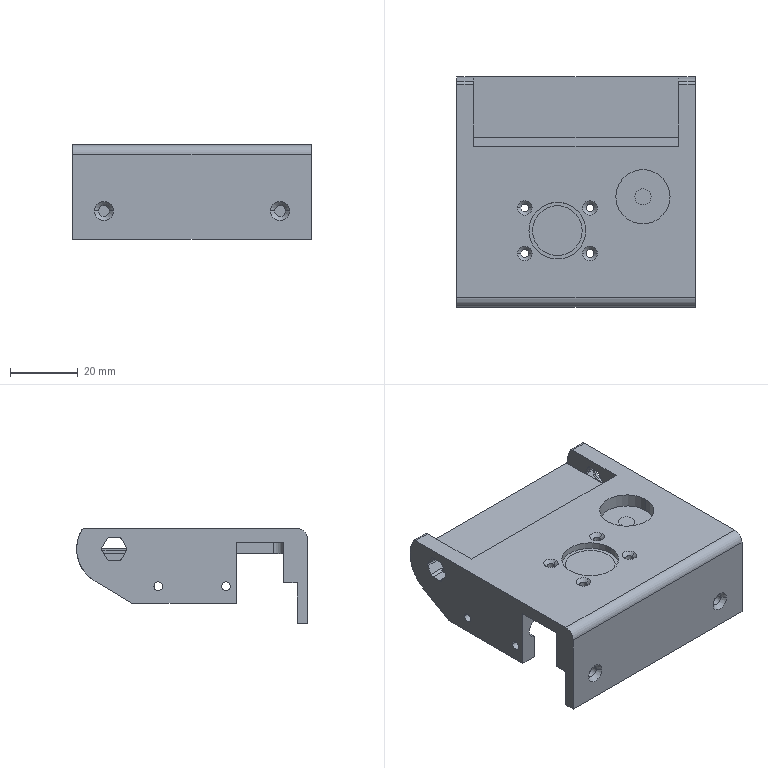NC program | NX | posted with a generic post | part box 70.5 x 68.1 x 28 mm
Whole program:
N10 G17 G21 G94 G90
(DRILLING_COPY_1 , TOOL : D6A45)
N12 T07 M6
N14 G54
N16 G17 G0 G90 X-24. Y-17. B0. C0. S3500 M3
N18 G43 Z30. H7
N20 G94 G81 G98 Z-1.4 F250. R3.
N22 X-44.
N24 G80
N26 G0 X-44. Y-17. Z30.
N28 M5
(DRILLING_COPY_COPY_COPY_1 , TOOL : 2.6ZT)
N30 T12 M6
N32 G54
N34 G17 G0 G90 X-24. Y-17. B0. C0. S2500 M3
N36 G43 Z30. H12
N38 G94 G83 G98 Z-7.281 F120. Q2. R3.
N40 X-44.
N42 G80
N44 G0 X-44. Y-17. Z30.
N46 M5
(ZLEVEL_PROFILE_COPY , TOOL : D2)
N48 T02 M6
N50 G54
N52 G17 G0 G90 X-55.895 Y-3.6 B0. C0. S9500 M3
N54 G43 Z30. H2
N56 Z1.
N58 G94 G1 X-58.386 Z0.869 F1000.
N60 X-59.769 Y-5.996 Z0.724
N62 X-59.764 Y-5.999
N64 X-59.765 Y-6.012
N66 X-58.388 Y-8.396 Z0.579
N68 X-58.379 Y-8.4
N70 X-55.614 Z0.434
N72 X-54.232 Y-6.006 Z0.289
N74 X-54.231 Y-5.996 Z0.288
N76 X-55.614 Y-3.6 Z0.143
N78 X-58.386 Z-0.002
N80 X-59.769 Y-5.996 Z-0.147
N82 X-59.764 Y-5.999
N84 X-59.765 Y-6.012
N86 X-58.388 Y-8.396
N88 X-58.379 Y-8.4
N90 X-55.614
N92 X-54.232 Y-6.006
N94 X-54.231 Y-5.996
N96 X-55.614 Y-3.6
N98 X-58.386
N100 X-59.769 Y-5.996
N102 X-59.764 Y-5.999
N104 X-59.721 Y-6.087 Z-0.149
N106 X-59.673 Y-6.17 Z-0.15
N108 X-58.448 Y-8.291 Z-0.193
N110 X-58.396 Y-8.374 Z-0.195
N112 X-58.376 Y-8.394
N114 X-58.216 Y-8.4 Z-0.198
N116 X-55.669 Z-0.243
N118 X-55.619 Y-8.393 Z-0.244
N120 X-55.543 Y-8.277 Z-0.246
N122 X-54.27 Y-6.071 Z-0.291
N124 X-54.248 Y-6.029 Z-0.292
N126 X-54.237 Y-5.986
N128 X-54.286 Y-5.9 Z-0.294
N130 X-55.614 Y-3.6
N132 X-58.386
N134 X-59.769 Y-5.996
N136 X-59.764 Y-5.999
N138 X-59.721 Y-6.087 Z-0.296
N140 X-59.673 Y-6.17 Z-0.298
N142 X-58.448 Y-8.291 Z-0.34
N144 X-58.396 Y-8.374 Z-0.342
N146 X-58.376 Y-8.394 Z-0.343
N148 X-58.216 Y-8.4 Z-0.345
N150 X-55.669 Z-0.39
N152 X-55.619 Y-8.393 Z-0.391
N154 X-55.543 Y-8.277 Z-0.393
N156 X-54.27 Y-6.071 Z-0.438
N158 X-54.248 Y-6.029 Z-0.439
N160 X-54.237 Y-5.986
N162 X-54.286 Y-5.9 Z-0.441
N164 X-55.614 Y-3.6
N166 X-58.386
N168 X-59.769 Y-5.996
N170 X-59.764 Y-5.999
N172 X-59.721 Y-6.087 Z-0.443
N174 X-59.673 Y-6.17 Z-0.445
N176 X-58.448 Y-8.291 Z-0.487
N178 X-58.396 Y-8.374 Z-0.489
N180 X-58.376 Y-8.394 Z-0.49
N182 X-58.216 Y-8.4 Z-0.492
N184 X-55.669 Z-0.537
N186 X-55.619 Y-8.392 Z-0.538
N188 X-55.543 Y-8.277 Z-0.54
N190 X-54.27 Y-6.071 Z-0.585
N192 X-54.248 Y-6.029 Z-0.586
N194 X-54.237 Y-5.986 Z-0.587
N196 X-54.286 Y-5.9 Z-0.588
N198 X-55.614 Y-3.6
N200 X-58.386
N202 X-59.769 Y-5.996
N204 X-59.764 Y-5.999
N206 X-59.721 Y-6.087 Z-0.59
N208 X-59.673 Y-6.17 Z-0.592
N210 X-58.448 Y-8.291 Z-0.634
N212 X-58.396 Y-8.374 Z-0.636
N214 X-58.376 Y-8.394 Z-0.637
N216 X-58.216 Y-8.4 Z-0.64
N218 X-55.669 Z-0.684
N220 X-55.619 Y-8.392 Z-0.685
N222 X-55.543 Y-8.277 Z-0.687
N224 X-54.27 Y-6.071 Z-0.732
N226 X-54.248 Y-6.029 Z-0.733
N228 X-54.237 Y-5.986 Z-0.734
N230 X-54.286 Y-5.9 Z-0.735
N232 X-55.614 Y-3.6
N234 X-58.386
N236 X-59.769 Y-5.996
N238 X-59.764 Y-5.999
N240 X-59.721 Y-6.087 Z-0.737
N242 X-59.673 Y-6.17 Z-0.739
N244 X-58.448 Y-8.291 Z-0.781
N246 X-58.396 Y-8.374 Z-0.783
N248 X-58.376 Y-8.394 Z-0.784
N250 X-58.216 Y-8.4 Z-0.787
N252 X-55.669 Z-0.831
N254 X-55.619 Y-8.392 Z-0.832
N256 X-55.543 Y-8.277 Z-0.834
N258 X-54.27 Y-6.071 Z-0.879
N260 X-54.248 Y-6.029 Z-0.88
N262 X-54.237 Y-5.986 Z-0.881
N264 X-54.286 Y-5.9 Z-0.882
N266 X-55.614 Y-3.6
N268 X-58.386
N270 X-59.769 Y-5.996
N272 X-59.764 Y-5.999
N274 X-59.721 Y-6.087 Z-0.884
N276 X-59.673 Y-6.17 Z-0.886
N278 X-58.448 Y-8.291 Z-0.929
N280 X-58.396 Y-8.374 Z-0.93
N282 X-58.376 Y-8.394 Z-0.931
N284 X-58.216 Y-8.4 Z-0.934
N286 X-55.669 Z-0.978
N288 X-55.619 Y-8.392 Z-0.979
N290 X-55.543 Y-8.277 Z-0.982
N292 X-54.27 Y-6.071 Z-1.026
N294 X-54.248 Y-6.029 Z-1.027
N296 X-54.237 Y-5.986 Z-1.028
N298 X-54.286 Y-5.9 Z-1.029
N300 X-55.614 Y-3.6
N302 X-58.386
N304 X-59.769 Y-5.996
N306 X-59.764 Y-5.999
N308 X-59.721 Y-6.087 Z-1.031
N310 X-59.673 Y-6.17 Z-1.033
N312 X-58.448 Y-8.291 Z-1.076
N314 X-58.396 Y-8.374 Z-1.077
N316 X-58.376 Y-8.394 Z-1.078
N318 X-58.216 Y-8.4 Z-1.081
N320 X-55.669 Z-1.125
N322 X-55.619 Y-8.392 Z-1.126
N324 X-55.543 Y-8.277 Z-1.129
N326 X-54.27 Y-6.071 Z-1.173
N328 X-54.248 Y-6.029 Z-1.174
N330 X-54.237 Y-5.986 Z-1.175
N332 X-54.286 Y-5.9 Z-1.176
N334 X-55.614 Y-3.6
N336 X-58.386
N338 X-59.769 Y-5.996
N340 X-59.764 Y-5.999
N342 X-59.721 Y-6.087 Z-1.178
N344 X-59.673 Y-6.17 Z-1.18
N346 X-58.448 Y-8.291 Z-1.223
N348 X-58.396 Y-8.374 Z-1.224
N350 X-58.376 Y-8.394 Z-1.225
N352 X-58.216 Y-8.4 Z-1.228
N354 X-55.669 Z-1.272
N356 X-55.619 Y-8.392 Z-1.273
N358 X-55.543 Y-8.277 Z-1.276
N360 X-54.27 Y-6.071 Z-1.32
N362 X-54.248 Y-6.029 Z-1.321
N364 X-54.237 Y-5.986 Z-1.322
N366 X-54.286 Y-5.9 Z-1.324
N368 X-55.614 Y-3.6
N370 X-58.386
N372 X-59.769 Y-5.996
N374 X-59.764 Y-5.999
N376 X-59.721 Y-6.087 Z-1.325
N378 X-59.673 Y-6.17 Z-1.327
N380 X-58.448 Y-8.291 Z-1.37
N382 X-58.396 Y-8.374 Z-1.371
N384 X-58.376 Y-8.394 Z-1.372
N386 X-58.216 Y-8.4 Z-1.375
N388 X-55.669 Z-1.419
N390 X-55.619 Y-8.392 Z-1.42
N392 X-55.543 Y-8.277 Z-1.423
N394 X-54.27 Y-6.071 Z-1.467
N396 X-54.248 Y-6.029 Z-1.468
N398 X-54.237 Y-5.986 Z-1.469
N400 X-54.286 Y-5.9 Z-1.471
N402 X-55.614 Y-3.6
N404 X-58.386
N406 X-59.769 Y-5.996
N408 X-59.764 Y-5.999
N410 X-59.721 Y-6.087 Z-1.472
N412 X-59.673 Y-6.17 Z-1.474
N414 X-58.448 Y-8.291 Z-1.517
N416 X-58.396 Y-8.374 Z-1.518
N418 X-58.376 Y-8.394 Z-1.519
N420 X-58.216 Y-8.4 Z-1.522
N422 X-55.669 Z-1.566
N424 X-55.619 Y-8.392 Z-1.567
N426 X-55.543 Y-8.277 Z-1.57
N428 X-54.27 Y-6.071 Z-1.614
N430 X-54.248 Y-6.029 Z-1.615
N432 X-54.237 Y-5.986 Z-1.616
N434 X-54.287 Y-5.9 Z-1.618
N436 X-55.614 Y-3.6
N438 X-58.386
N440 X-59.769 Y-5.996
N442 X-59.764 Y-5.999
N444 X-59.721 Y-6.087 Z-1.619
N446 X-59.673 Y-6.17 Z-1.621
N448 X-58.448 Y-8.291 Z-1.664
N450 X-58.396 Y-8.374 Z-1.666
N452 X-58.376 Y-8.393
N454 X-58.216 Y-8.4 Z-1.669
N456 X-55.669 Z-1.713
N458 X-55.619 Y-8.392 Z-1.714
N460 X-55.543 Y-8.277 Z-1.717
N462 X-54.27 Y-6.071 Z-1.761
N464 X-54.248 Y-6.029 Z-1.762
N466 X-54.237 Y-5.986 Z-1.763
N468 X-54.287 Y-5.9 Z-1.765
N470 X-55.614 Y-3.6
N472 X-58.386
N474 X-59.769 Y-5.996
N476 X-59.764 Y-5.999
N478 X-59.721 Y-6.087 Z-1.766
N480 X-59.673 Y-6.17 Z-1.768
N482 X-58.448 Y-8.291 Z-1.811
N484 X-58.396 Y-8.374 Z-1.813
N486 X-58.376 Y-8.393
N488 X-58.216 Y-8.4 Z-1.816
N490 X-55.669 Z-1.86
N492 X-55.619 Y-8.392 Z-1.861
N494 X-55.543 Y-8.277 Z-1.864
N496 X-54.27 Y-6.071 Z-1.908
N498 X-54.248 Y-6.029 Z-1.909
N500 X-54.237 Y-5.986 Z-1.91
N502 X-54.287 Y-5.9 Z-1.912
N504 X-55.614 Y-3.6
N506 X-58.386
N508 X-59.769 Y-5.996
N510 X-59.764 Y-5.999
N512 X-59.721 Y-6.087 Z-1.913
N514 X-59.673 Y-6.17 Z-1.915
N516 X-58.448 Y-8.291 Z-1.958
N518 X-58.396 Y-8.374 Z-1.96
N520 X-58.376 Y-8.393
N522 X-58.216 Y-8.4 Z-1.963
N524 X-55.669 Z-2.008
N526 X-55.619 Y-8.392
N528 X-55.543 Y-8.277 Z-2.011
N530 X-54.27 Y-6.071 Z-2.055
N532 X-54.248 Y-6.029 Z-2.056
N534 X-54.237 Y-5.986 Z-2.057
N536 X-54.287 Y-5.9 Z-2.059
N538 X-55.614 Y-3.6
N540 X-58.386
N542 X-59.769 Y-5.996
N544 X-59.764 Y-5.999
N546 X-59.721 Y-6.087 Z-2.061
N548 X-59.673 Y-6.17 Z-2.062
N550 X-58.448 Y-8.291 Z-2.105
N552 X-58.396 Y-8.374 Z-2.107
N554 X-58.376 Y-8.393
N556 X-58.216 Y-8.4 Z-2.11
N558 X-55.669 Z-2.155
N560 X-55.619 Y-8.392 Z-2.156
N562 X-55.543 Y-8.277 Z-2.158
N564 X-54.27 Y-6.071 Z-2.202
N566 X-54.248 Y-6.029 Z-2.203
N568 X-54.237 Y-5.986 Z-2.204
N570 X-54.287 Y-5.9 Z-2.206
N572 X-55.614 Y-3.6
N574 X-58.386
N576 X-59.769 Y-5.996
N578 X-59.764 Y-5.999
N580 X-59.721 Y-6.087 Z-2.208
N582 X-59.673 Y-6.17 Z-2.209
N584 X-58.448 Y-8.291 Z-2.252
N586 X-58.396 Y-8.374 Z-2.254
N588 X-58.376 Y-8.393
N590 X-58.216 Y-8.4 Z-2.257
N592 X-55.669 Z-2.302
N594 X-55.619 Y-8.392 Z-2.303
N596 X-55.543 Y-8.277 Z-2.305
N598 X-54.27 Y-6.071 Z-2.35
N600 X-54.248 Y-6.029
N602 X-54.237 Y-5.986 Z-2.351
N604 X-54.287 Y-5.9 Z-2.353
N606 X-55.614 Y-3.6
N608 X-58.386
N610 X-59.769 Y-5.996
N612 X-59.764 Y-5.999
N614 X-59.721 Y-6.087 Z-2.355
N616 X-59.673 Y-6.17 Z-2.356
N618 X-58.448 Y-8.291 Z-2.399
N620 X-58.396 Y-8.374 Z-2.401
N622 X-58.376 Y-8.393
N624 X-58.216 Y-8.4 Z-2.404
N626 X-55.669 Z-2.449
N628 X-55.619 Y-8.392 Z-2.45
N630 X-55.543 Y-8.277 Z-2.452
N632 X-54.27 Y-6.071 Z-2.497
N634 X-54.248 Y-6.029
N636 X-54.237 Y-5.986 Z-2.498
N638 X-54.287 Y-5.9 Z-2.5
N640 X-55.614 Y-3.6
N642 X-58.386
N644 X-59.769 Y-5.996
N646 X-59.764 Y-5.999
N648 X-59.721 Y-6.087 Z-2.502
N650 X-59.673 Y-6.17 Z-2.503
N652 X-58.448 Y-8.291 Z-2.546
N654 X-58.396 Y-8.374 Z-2.548
N656 X-58.376 Y-8.393
N658 X-58.216 Y-8.4 Z-2.551
N660 X-55.669 Z-2.596
N662 X-55.619 Y-8.392 Z-2.597
N664 X-55.543 Y-8.277 Z-2.599
N666 X-54.27 Y-6.071 Z-2.644
N668 X-54.248 Y-6.029
N670 X-54.237 Y-5.986 Z-2.645
N672 X-54.287 Y-5.9 Z-2.647
N674 X-55.614 Y-3.6
N676 X-58.386
N678 X-59.769 Y-5.996
N680 X-59.764 Y-5.999
N682 X-59.721 Y-6.087 Z-2.649
N684 X-59.673 Y-6.17 Z-2.65
N686 X-58.448 Y-8.291 Z-2.693
N688 X-58.396 Y-8.374 Z-2.695
N690 X-58.376 Y-8.393
N692 X-58.216 Y-8.4 Z-2.698
N694 X-55.669 Z-2.743
N696 X-55.619 Y-8.392 Z-2.744
N698 X-55.543 Y-8.277 Z-2.746
N700 X-54.27 Y-6.071 Z-2.791
N702 X-54.248 Y-6.029 Z-2.792
N704 X-54.237 Y-5.986
N706 X-54.287 Y-5.9 Z-2.794
N708 X-55.614 Y-3.6
N710 X-58.386
N712 X-59.769 Y-5.996
N714 X-59.764 Y-5.999
N716 X-59.721 Y-6.087 Z-2.796
N718 X-59.673 Y-6.17 Z-2.798
N720 X-58.448 Y-8.291 Z-2.84
N722 X-58.396 Y-8.374 Z-2.842
N724 X-58.376 Y-8.393 Z-2.843
N726 X-58.216 Y-8.4 Z-2.845
N728 X-55.669 Z-2.89
N730 X-55.619 Y-8.392 Z-2.891
N732 X-55.543 Y-8.277 Z-2.893
N734 X-54.27 Y-6.071 Z-2.938
N736 X-54.248 Y-6.029 Z-2.939
N738 X-54.237 Y-5.986
N740 X-54.287 Y-5.9 Z-2.941
N742 X-55.614 Y-3.6
N744 X-58.386
N746 X-59.769 Y-5.996
N748 X-59.764 Y-5.999
N750 X-59.721 Y-6.087 Z-2.943
N752 X-59.673 Y-6.17 Z-2.945
N754 X-58.448 Y-8.291 Z-2.987
N756 X-58.396 Y-8.374 Z-2.989
N758 X-58.376 Y-8.393 Z-2.99
N760 X-58.216 Y-8.4 Z-2.992
N762 X-55.669 Z-3.037
N764 X-55.619 Y-8.392 Z-3.038
N766 X-55.543 Y-8.277 Z-3.04
N768 X-54.27 Y-6.071 Z-3.085
N770 X-54.248 Y-6.029 Z-3.086
N772 X-54.237 Y-5.986 Z-3.087
N774 X-54.287 Y-5.9 Z-3.088
N776 X-55.614 Y-3.6
N778 X-58.386
N780 X-59.769 Y-5.996
N782 X-59.764 Y-5.999
N784 X-59.721 Y-6.087 Z-3.09
N786 X-59.673 Y-6.17 Z-3.092
N788 X-58.448 Y-8.291 Z-3.134
N790 X-58.396 Y-8.374 Z-3.136
N792 X-58.376 Y-8.393 Z-3.137
N794 X-58.216 Y-8.4 Z-3.14
N796 X-55.669 Z-3.184
N798 X-55.619 Y-8.392 Z-3.185
N800 X-55.543 Y-8.277 Z-3.187
N802 X-54.27 Y-6.071 Z-3.232
N804 X-54.248 Y-6.029 Z-3.233
N806 X-54.237 Y-5.986 Z-3.234
N808 X-54.287 Y-5.9 Z-3.235
N810 X-55.614 Y-3.6
N812 X-58.386
N814 X-59.769 Y-5.996
N816 X-59.764 Y-5.999
N818 X-59.721 Y-6.087 Z-3.237
N820 X-59.673 Y-6.17 Z-3.239
N822 X-58.448 Y-8.291 Z-3.281
N824 X-58.396 Y-8.374 Z-3.283
N826 X-58.376 Y-8.393 Z-3.284
N828 X-58.216 Y-8.4 Z-3.287
N830 X-55.669 Z-3.331
N832 X-55.619 Y-8.392 Z-3.332
N834 X-55.543 Y-8.277 Z-3.334
N836 X-54.27 Y-6.071 Z-3.379
N838 X-54.248 Y-6.029 Z-3.38
N840 X-54.237 Y-5.986 Z-3.381
N842 X-54.287 Y-5.9 Z-3.382
N844 X-55.614 Y-3.6
N846 X-58.386
N848 X-59.769 Y-5.996
N850 X-59.764 Y-5.999
N852 X-59.721 Y-6.087 Z-3.384
N854 X-59.673 Y-6.17 Z-3.386
N856 X-58.448 Y-8.291 Z-3.429
N858 X-58.396 Y-8.374 Z-3.43
N860 X-58.376 Y-8.393 Z-3.431
N862 X-58.216 Y-8.4 Z-3.434
N864 X-55.669 Z-3.478
N866 X-55.619 Y-8.391 Z-3.479
N868 X-55.59 Y-8.358 Z-3.48
N870 X-55.542 Y-8.274 Z-3.482
N872 X-54.268 Y-6.068 Z-3.526
N874 X-54.247 Y-6.025 Z-3.527
N876 X-54.239 Y-5.982 Z-3.528
N878 X-54.288 Y-5.897 Z-3.529
N880 X-55.614 Y-3.6
N882 X-58.386
N884 X-59.769 Y-5.996
N886 X-59.764 Y-5.999
N888 X-59.721 Y-6.087 Z-3.531
N890 X-59.673 Y-6.17 Z-3.533
N892 X-58.448 Y-8.291 Z-3.576
N894 X-58.396 Y-8.374 Z-3.577
N896 X-58.376 Y-8.393 Z-3.578
N898 X-58.216 Y-8.4 Z-3.581
N900 X-55.669 Z-3.625
N902 X-55.619 Y-8.391 Z-3.626
N904 X-55.59 Y-8.358 Z-3.627
N906 X-55.542 Y-8.274 Z-3.629
N908 X-54.268 Y-6.068 Z-3.673
N910 X-54.247 Y-6.025 Z-3.674
N912 X-54.239 Y-5.982 Z-3.675
N914 X-54.288 Y-5.897 Z-3.676
N916 X-55.614 Y-3.6
N918 X-58.386
N920 X-59.769 Y-5.996
N922 X-59.764 Y-5.999
N924 X-59.721 Y-6.087 Z-3.678
N926 X-59.673 Y-6.17 Z-3.68
N928 X-58.448 Y-8.291 Z-3.723
N930 X-58.396 Y-8.374 Z-3.724
N932 X-58.376 Y-8.393 Z-3.725
N934 X-58.216 Y-8.4 Z-3.728
N936 X-55.669 Z-3.772
N938 X-55.619 Y-8.391 Z-3.773
N940 X-55.59 Y-8.358 Z-3.774
N942 X-55.542 Y-8.274 Z-3.776
N944 X-54.268 Y-6.068 Z-3.82
N946 X-54.247 Y-6.025 Z-3.821
N948 X-54.239 Y-5.982 Z-3.822
N950 X-54.288 Y-5.897 Z-3.824
N952 X-55.614 Y-3.6
N954 X-58.386
N956 X-59.769 Y-5.996
N958 X-59.764 Y-5.999
N960 X-59.721 Y-6.087 Z-3.825
N962 X-59.673 Y-6.17 Z-3.827
N964 X-58.448 Y-8.291 Z-3.87
N966 X-58.396 Y-8.374 Z-3.871
N968 X-58.375 Y-8.393 Z-3.872
N970 X-58.216 Y-8.4 Z-3.875
N972 X-55.669 Z-3.919
N974 X-55.619 Y-8.391 Z-3.92
N976 X-55.59 Y-8.358 Z-3.921
N978 X-55.542 Y-8.274 Z-3.923
N980 X-54.268 Y-6.068 Z-3.967
N982 X-54.247 Y-6.025 Z-3.968
N984 X-54.239 Y-5.982 Z-3.969
N986 X-54.288 Y-5.897 Z-3.971
N988 X-55.614 Y-3.6
N990 X-58.386
N992 X-59.769 Y-5.996
N994 X-59.764 Y-5.999
N996 X-59.721 Y-6.087 Z-3.972
N998 X-59.673 Y-6.17 Z-3.974
N1000 X-58.448 Y-8.291 Z-4.017
N1002 X-58.396 Y-8.374 Z-4.018
N1004 X-58.375 Y-8.393 Z-4.019
N1006 X-58.215 Y-8.4 Z-4.022
N1008 X-55.668 Z-4.066
N1010 X-55.619 Y-8.391 Z-4.067
N1012 X-55.591 Y-8.359 Z-4.068
N1014 X-55.543 Y-8.276 Z-4.07
N1016 X-54.269 Y-6.07 Z-4.114
N1018 X-54.248 Y-6.027 Z-4.115
N1020 X-54.238 Y-5.984 Z-4.116
N1022 X-54.287 Y-5.898 Z-4.118
N1024 X-55.614 Y-3.6
N1026 X-58.386
N1028 X-59.769 Y-5.996
N1030 X-59.764 Y-5.999
N1032 X-59.721 Y-6.087 Z-4.119
N1034 X-59.673 Y-6.17 Z-4.121
N1036 X-58.448 Y-8.291 Z-4.164
N1038 X-58.396 Y-8.374 Z-4.166
N1040 X-58.375 Y-8.393
N1042 X-58.215 Y-8.4 Z-4.169
N1044 X-55.668 Z-4.213
N1046 X-55.619 Y-8.391 Z-4.214
N1048 X-55.591 Y-8.359 Z-4.215
N1050 X-55.543 Y-8.276 Z-4.217
N1052 X-54.269 Y-6.07 Z-4.261
N1054 X-54.248 Y-6.027 Z-4.262
N1056 X-54.238 Y-5.984 Z-4.263
N1058 X-54.287 Y-5.899 Z-4.265
N1060 X-55.614 Y-3.6
N1062 X-58.386
N1064 X-59.769 Y-5.996
N1066 X-59.764 Y-5.999
N1068 X-59.721 Y-6.087 Z-4.266
N1070 X-59.673 Y-6.17 Z-4.268
N1072 X-58.448 Y-8.291 Z-4.311
N1074 X-58.396 Y-8.374 Z-4.313
N1076 X-58.375 Y-8.393
N1078 X-58.215 Y-8.4 Z-4.316
N1080 X-55.668 Z-4.36
N1082 X-55.619 Y-8.391 Z-4.361
N1084 X-55.591 Y-8.359 Z-4.362
N1086 X-55.543 Y-8.276 Z-4.364
N1088 X-54.269 Y-6.07 Z-4.408
N1090 X-54.248 Y-6.027 Z-4.409
N1092 X-54.238 Y-5.984 Z-4.41
N1094 X-54.287 Y-5.899 Z-4.412
N1096 X-55.614 Y-3.6
N1098 X-58.386
N1100 X-59.769 Y-5.996
N1102 X-59.764 Y-5.999
N1104 X-59.721 Y-6.087 Z-4.413
N1106 X-59.673 Y-6.17 Z-4.415
N1108 X-58.448 Y-8.291 Z-4.458
N1110 X-58.396 Y-8.374 Z-4.46
N1112 X-58.375 Y-8.393
N1114 X-58.215 Y-8.4 Z-4.463
N1116 X-55.668 Z-4.508
N1118 X-55.619 Y-8.391
N1120 X-55.591 Y-8.359 Z-4.509
N1122 X-55.543 Y-8.276 Z-4.511
N1124 X-54.269 Y-6.07 Z-4.555
N1126 X-54.248 Y-6.027 Z-4.556
N1128 X-54.238 Y-5.985 Z-4.557
N1130 X-54.287 Y-5.899 Z-4.559
N1132 X-55.614 Y-3.6
N1134 X-58.386
N1136 X-59.769 Y-5.996
N1138 X-59.764 Y-5.999
N1140 X-59.721 Y-6.087 Z-4.561
N1142 X-59.673 Y-6.17 Z-4.562
N1144 X-58.448 Y-8.291 Z-4.605
N1146 X-58.396 Y-8.374 Z-4.607
N1148 X-58.375 Y-8.393
N1150 X-58.215 Y-8.4 Z-4.61
N1152 X-55.668 Z-4.655
N1154 X-55.62 Y-8.39 Z-4.656
N1156 X-55.591 Y-8.359
N1158 X-55.543 Y-8.276 Z-4.658
N1160 X-54.269 Y-6.07 Z-4.702
N1162 X-54.248 Y-6.028 Z-4.703
N1164 X-54.238 Y-5.985 Z-4.704
N1166 X-54.287 Y-5.899 Z-4.706
N1168 X-55.614 Y-3.6
N1170 X-58.386
N1172 X-59.769 Y-5.996
N1174 X-59.764 Y-5.999
N1176 X-59.721 Y-6.087 Z-4.708
N1178 X-59.673 Y-6.17 Z-4.709
N1180 X-58.448 Y-8.291 Z-4.752
N1182 X-58.396 Y-8.374 Z-4.754
N1184 X-58.379 Y-8.394
N1186 X-58.215 Y-8.397 Z-4.757
N1188 X-57.922 Y-8.398 Z-4.762
N1190 X-57.824 Y-8.4 Z-4.764
N1192 X-56.256 Z-4.791
N1194 X-56.158 Z-4.793
N1196 X-56.06 Y-8.399 Z-4.795
N1198 X-55.962 Z-4.797
N1200 X-55.864 Z-4.798
N1202 X-55.766 Y-8.4 Z-4.8
N1204 X-55.668 Y-8.394 Z-4.802
N1206 X-55.616 Y-8.379 Z-4.803
N1208 X-55.587 Y-8.353
N1210 X-55.543 Y-8.277 Z-4.805
N1212 X-54.27 Y-6.071 Z-4.85
N1214 X-54.248 Y-6.028
N1216 X-54.237 Y-5.985 Z-4.851
N1218 X-54.287 Y-5.9 Z-4.853
N1220 X-55.614 Y-3.6
N1222 X-58.386
N1224 X-59.769 Y-5.996
N1226 X-59.764 Y-5.999
N1228 X-59.721 Y-6.087 Z-4.855
N1230 X-59.673 Y-6.17 Z-4.856
N1232 X-58.448 Y-8.291 Z-4.899
N1234 X-58.396 Y-8.374 Z-4.901
N1236 X-58.381 Y-8.394
N1238 X-58.215 Y-8.396 Z-4.904
N1240 X-58.118 Y-8.397 Z-4.906
N1242 X-58.02 Z-4.908
N1244 X-57.922 Z-4.909
N1246 X-57.824 Z-4.911
N1248 X-57.726 Y-8.398 Z-4.913
N1250 X-57.628 Z-4.915
N1252 X-57.53 Y-8.399 Z-4.916
N1254 X-57.432 Z-4.918
N1256 X-57.334 Z-4.92
N1258 X-57.236 Y-8.4 Z-4.921
N1260 X-56.256 Z-4.938
N1262 X-56.158 Z-4.94
N1264 X-56.06 Y-8.399 Z-4.942
N1266 X-55.962 Z-4.944
N1268 X-55.864 Z-4.945
N1270 X-55.692 Y-8.39 Z-4.948
N1272 X-55.591 Y-8.36 Z-4.95
N1274 X-55.538 Y-8.267 Z-4.952
N1276 X-54.264 Y-6.062 Z-4.997
N1278 X-54.245 Y-6.019
N1280 X-54.243 Y-5.976 Z-4.998
N1282 X-54.292 Y-5.89 Z-5.
N1284 X-55.614 Y-3.6
N1286 X-58.386
N1288 X-59.769 Y-5.996
N1290 X-59.764 Y-5.999
N1292 Y-6.012
N1294 X-58.388 Y-8.396
N1296 X-58.376 Y-8.4
N1298 X-58.344
N1300 X-55.798
N1302 G3 X-55.594 Y-8.365 R0.624
N1304 G1 X-54.233 Y-6.007
N1306 Y-5.992
N1308 X-54.292 Y-5.89
N1310 Z-4.
N1312 G0 Z30.
N1314 M5
(ZLEVEL_PROFILE_1_COPY_1_COPY_COPY_COPY_1_COPY_COPY , TOOL : D6A45)
N1316 T07 M6
N1318 G54
N1320 G17 G0 G90 X-44. Y-17.341 B0. C0. S9500 M3
N1322 G43 Z30. H7
N1324 Z1.
N1326 G94 G1 Z-1. F1000.
N1328 G3 X-43.659 Y-17. R0.341
N1330 X-44. Y-17.341 R-0.341
N1332 X-43.74 Y-17.191 R0.3
N1334 G1 Z0.
N1336 G0 Z30.
N1338 X-24. Y-17.341
N1340 Z1.
N1342 G1 Z-1.
N1344 G3 X-23.659 Y-17. R0.341
N1346 X-24. Y-17.341 R-0.341
N1348 X-23.74 Y-17.191 R0.3
N1350 G1 Z0.
N1352 G0 Z30.
N1354 X-55.728 Y-6.279
N1356 Z0.
N1358 G1 Z-1.
N1360 X-54.712
N1362 G3 X-54.193 Y-5.979 R0.6
N1364 G1 X-55.578 Y-3.579
N1366 X-55.589 Y-3.555
N1368 X-55.614 Y-3.559
N1370 X-58.386
N1372 X-58.411 Y-3.555
N1374 X-58.422 Y-3.579
N1376 X-59.807 Y-5.979
N1378 X-59.823 Y-6.
N1380 X-59.807 Y-6.021
N1382 X-58.422 Y-8.421
N1384 X-58.411 Y-8.445
N1386 X-58.386 Y-8.441
N1388 X-55.614
N1390 X-55.589 Y-8.445
N1392 X-55.578 Y-8.421
N1394 X-54.193 Y-6.021
N1396 X-54.177 Y-6.
N1398 X-54.193 Y-5.979
N1400 G3 X-54.712 Y-5.679 R0.6
N1402 G1 X-55.752
N1404 Z0.
N1406 G0 Z30.
N1408 M5
N1410 M2